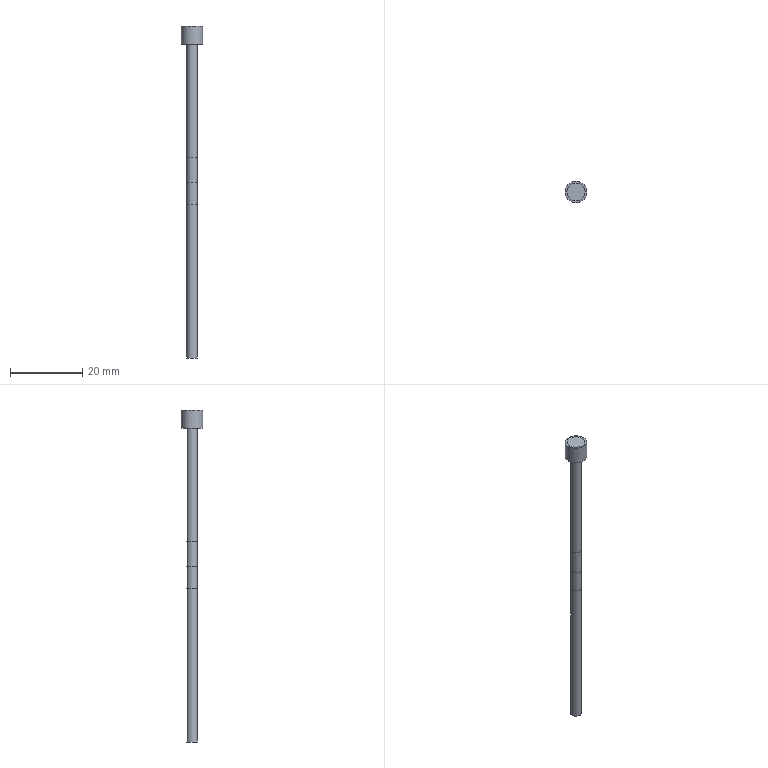Part | NX | features BREP 3 | 3 solids | 17 faces | box 6 x 6 x 92.2 mm | volume 1282 mm3 | plane 9 | cylinder 7 | torus 1 | commonest cylinder face diameters 3 x3 2 x1 2.1 x1 5 x1 6 x1
STEP:
#1=CARTESIAN_POINT('',(-1.5,0.,15.4));
#2=VERTEX_POINT('',#1);
#3=CARTESIAN_POINT('',(0.,0.,15.4));
#4=DIRECTION('',(0.,0.,-1.));
#5=DIRECTION('',(-1.,0.,0.));
#6=AXIS2_PLACEMENT_3D('',#3,#4,#5);
#7=CIRCLE('',#6,1.5);
#8=EDGE_CURVE('',#2,#2,#7,.T.);
#9=ORIENTED_EDGE('',*,*,#8,.T.);
#10=EDGE_LOOP('',(#9));
#11=FACE_BOUND('',#10,.T.);
#12=CARTESIAN_POINT('',(-1.5,0.,-40.2));
#13=VERTEX_POINT('',#12);
#14=CARTESIAN_POINT('',(0.,0.,-40.2));
#15=DIRECTION('',(0.,0.,-1.));
#16=DIRECTION('',(-1.,0.,0.));
#17=AXIS2_PLACEMENT_3D('',#14,#15,#16);
#18=CIRCLE('',#17,1.5);
#19=EDGE_CURVE('',#13,#13,#18,.T.);
#20=ORIENTED_EDGE('',*,*,#19,.F.);
#21=EDGE_LOOP('',(#20));
#22=FACE_BOUND('',#21,.T.);
#23=CARTESIAN_POINT('',(0.,0.,15.4));
#24=DIRECTION('',(0.,0.,-1.));
#25=DIRECTION('',(1.,0.,0.));
#26=AXIS2_PLACEMENT_3D('',#23,#24,#25);
#27=CYLINDRICAL_SURFACE('',#26,1.5);
#28=ADVANCED_FACE('',(#11,#22),#27,.T.);
#29=ORIENTED_EDGE('',*,*,#8,.F.);
#30=EDGE_LOOP('',(#29));
#31=FACE_BOUND('',#30,.T.);
#32=CARTESIAN_POINT('',(0.,0.,15.4));
#33=DIRECTION('',(0.,0.,-1.));
#34=DIRECTION('',(1.,0.,0.));
#35=AXIS2_PLACEMENT_3D('',#32,#33,#34);
#36=PLANE('',#35);
#37=ADVANCED_FACE('',(#31),#36,.F.);
#38=ORIENTED_EDGE('',*,*,#19,.T.);
#39=EDGE_LOOP('',(#38));
#40=FACE_BOUND('',#39,.T.);
#41=CARTESIAN_POINT('',(0.,0.,-40.2));
#42=DIRECTION('',(0.,0.,-1.));
#43=DIRECTION('',(1.,0.,0.));
#44=AXIS2_PLACEMENT_3D('',#41,#42,#43);
#45=PLANE('',#44);
#46=ADVANCED_FACE('',(#40),#45,.T.);
#47=CLOSED_SHELL('',(#28,#37,#46));
#48=MANIFOLD_SOLID_BREP('',#47);
#49=CARTESIAN_POINT('',(2.5,0.,47.));
#50=VERTEX_POINT('',#49);
#51=CARTESIAN_POINT('',(0.,0.,47.));
#52=DIRECTION('',(0.,0.,-1.));
#53=DIRECTION('',(1.,0.,0.));
#54=AXIS2_PLACEMENT_3D('',#51,#52,#53);
#55=CIRCLE('',#54,2.5);
#56=EDGE_CURVE('',#50,#50,#55,.T.);
#57=ORIENTED_EDGE('',*,*,#56,.F.);
#58=EDGE_LOOP('',(#57));
#59=FACE_BOUND('',#58,.T.);
#60=CARTESIAN_POINT('',(2.5,0.,52.));
#61=VERTEX_POINT('',#60);
#62=CARTESIAN_POINT('',(0.,0.,52.));
#63=DIRECTION('',(0.,0.,-1.));
#64=DIRECTION('',(1.,0.,0.));
#65=AXIS2_PLACEMENT_3D('',#62,#63,#64);
#66=CIRCLE('',#65,2.5);
#67=EDGE_CURVE('',#61,#61,#66,.T.);
#68=ORIENTED_EDGE('',*,*,#67,.T.);
#69=EDGE_LOOP('',(#68));
#70=FACE_BOUND('',#69,.T.);
#71=CARTESIAN_POINT('',(0.,0.,47.));
#72=DIRECTION('',(0.,0.,1.));
#73=DIRECTION('',(-1.,0.,0.));
#74=AXIS2_PLACEMENT_3D('',#71,#72,#73);
#75=CYLINDRICAL_SURFACE('',#74,2.5);
#76=ADVANCED_FACE('',(#59,#70),#75,.T.);
#77=CARTESIAN_POINT('',(-1.5,0.,47.));
#78=VERTEX_POINT('',#77);
#79=CARTESIAN_POINT('',(0.,0.,47.));
#80=DIRECTION('',(0.,0.,-1.));
#81=DIRECTION('',(-1.,0.,0.));
#82=AXIS2_PLACEMENT_3D('',#79,#80,#81);
#83=CIRCLE('',#82,1.5);
#84=EDGE_CURVE('',#78,#78,#83,.T.);
#85=ORIENTED_EDGE('',*,*,#84,.F.);
#86=EDGE_LOOP('',(#85));
#87=FACE_BOUND('',#86,.T.);
#88=ORIENTED_EDGE('',*,*,#56,.T.);
#89=EDGE_LOOP('',(#88));
#90=FACE_BOUND('',#89,.T.);
#91=CARTESIAN_POINT('',(0.,0.,47.));
#92=DIRECTION('',(0.,0.,-1.));
#93=DIRECTION('',(1.,0.,0.));
#94=AXIS2_PLACEMENT_3D('',#91,#92,#93);
#95=PLANE('',#94);
#96=ADVANCED_FACE('',(#87,#90),#95,.T.);
#97=ORIENTED_EDGE('',*,*,#67,.F.);
#98=EDGE_LOOP('',(#97));
#99=FACE_BOUND('',#98,.T.);
#100=CARTESIAN_POINT('',(0.,0.,52.));
#101=DIRECTION('',(0.,0.,-1.));
#102=DIRECTION('',(1.,0.,0.));
#103=AXIS2_PLACEMENT_3D('',#100,#101,#102);
#104=PLANE('',#103);
#105=ADVANCED_FACE('',(#99),#104,.F.);
#106=ORIENTED_EDGE('',*,*,#84,.T.);
#107=EDGE_LOOP('',(#106));
#108=FACE_BOUND('',#107,.T.);
#109=CARTESIAN_POINT('',(-1.5,0.,8.522));
#110=VERTEX_POINT('',#109);
#111=CARTESIAN_POINT('',(0.,0.,8.522));
#112=DIRECTION('',(0.,0.,-1.));
#113=DIRECTION('',(-1.,0.,0.));
#114=AXIS2_PLACEMENT_3D('',#111,#112,#113);
#115=CIRCLE('',#114,1.5);
#116=EDGE_CURVE('',#110,#110,#115,.T.);
#117=ORIENTED_EDGE('',*,*,#116,.F.);
#118=EDGE_LOOP('',(#117));
#119=FACE_BOUND('',#118,.T.);
#120=CARTESIAN_POINT('',(0.,0.,47.));
#121=DIRECTION('',(0.,0.,-1.));
#122=DIRECTION('',(1.,0.,0.));
#123=AXIS2_PLACEMENT_3D('',#120,#121,#122);
#124=CYLINDRICAL_SURFACE('',#123,1.5);
#125=ADVANCED_FACE('',(#108,#119),#124,.T.);
#126=ORIENTED_EDGE('',*,*,#116,.T.);
#127=EDGE_LOOP('',(#126));
#128=FACE_BOUND('',#127,.T.);
#129=CARTESIAN_POINT('',(-1.,0.,5.4));
#130=VERTEX_POINT('',#129);
#131=CARTESIAN_POINT('',(0.,0.,5.4));
#132=DIRECTION('',(0.,0.,-1.));
#133=DIRECTION('',(-1.,0.,0.));
#134=AXIS2_PLACEMENT_3D('',#131,#132,#133);
#135=CIRCLE('',#134,1.);
#136=EDGE_CURVE('',#130,#130,#135,.T.);
#137=ORIENTED_EDGE('',*,*,#136,.F.);
#138=EDGE_LOOP('',(#137));
#139=FACE_BOUND('',#138,.T.);
#140=CARTESIAN_POINT('',(0.,0.,5.4));
#141=DIRECTION('',(0.,0.,-1.));
#142=DIRECTION('',(1.,0.,0.));
#143=AXIS2_PLACEMENT_3D('',#140,#141,#142);
#144=TOROIDAL_SURFACE('',#143,11.,10.);
#145=ADVANCED_FACE('',(#128,#139),#144,.F.);
#146=ORIENTED_EDGE('',*,*,#136,.T.);
#147=EDGE_LOOP('',(#146));
#148=FACE_BOUND('',#147,.T.);
#149=CARTESIAN_POINT('',(1.,0.,-3.6));
#150=VERTEX_POINT('',#149);
#151=CARTESIAN_POINT('',(0.,0.,-3.6));
#152=DIRECTION('',(0.,0.,1.));
#153=DIRECTION('',(1.,0.,0.));
#154=AXIS2_PLACEMENT_3D('',#151,#152,#153);
#155=CIRCLE('',#154,1.);
#156=EDGE_CURVE('',#150,#150,#155,.T.);
#157=ORIENTED_EDGE('',*,*,#156,.T.);
#158=EDGE_LOOP('',(#157));
#159=FACE_BOUND('',#158,.T.);
#160=CARTESIAN_POINT('',(0.,0.,0.));
#161=DIRECTION('',(0.,0.,1.));
#162=DIRECTION('',(-1.,0.,0.));
#163=AXIS2_PLACEMENT_3D('',#160,#161,#162);
#164=CYLINDRICAL_SURFACE('',#163,1.);
#165=ADVANCED_FACE('',(#148,#159),#164,.T.);
#166=ORIENTED_EDGE('',*,*,#156,.F.);
#167=EDGE_LOOP('',(#166));
#168=FACE_BOUND('',#167,.T.);
#169=CARTESIAN_POINT('',(5.458,-13.172,-3.6));
#170=DIRECTION('',(0.,0.,1.));
#171=DIRECTION('',(-1.,0.,0.));
#172=AXIS2_PLACEMENT_3D('',#169,#170,#171);
#173=PLANE('',#172);
#174=ADVANCED_FACE('',(#168),#173,.F.);
#175=CLOSED_SHELL('',(#76,#96,#105,#125,#145,#165,#174));
#176=MANIFOLD_SOLID_BREP('',#175);
#177=CARTESIAN_POINT('',(3.,0.,47.));
#178=VERTEX_POINT('',#177);
#179=CARTESIAN_POINT('',(0.,0.,47.));
#180=DIRECTION('',(0.,0.,-1.));
#181=DIRECTION('',(1.,0.,0.));
#182=AXIS2_PLACEMENT_3D('',#179,#180,#181);
#183=CIRCLE('',#182,3.);
#184=EDGE_CURVE('',#178,#178,#183,.T.);
#185=ORIENTED_EDGE('',*,*,#184,.F.);
#186=EDGE_LOOP('',(#185));
#187=FACE_BOUND('',#186,.T.);
#188=CARTESIAN_POINT('',(3.,0.,52.));
#189=VERTEX_POINT('',#188);
#190=CARTESIAN_POINT('',(0.,0.,52.));
#191=DIRECTION('',(0.,0.,-1.));
#192=DIRECTION('',(1.,0.,0.));
#193=AXIS2_PLACEMENT_3D('',#190,#191,#192);
#194=CIRCLE('',#193,3.);
#195=EDGE_CURVE('',#189,#189,#194,.T.);
#196=ORIENTED_EDGE('',*,*,#195,.T.);
#197=EDGE_LOOP('',(#196));
#198=FACE_BOUND('',#197,.T.);
#199=CARTESIAN_POINT('',(0.,0.,47.));
#200=DIRECTION('',(0.,0.,1.));
#201=DIRECTION('',(-1.,0.,0.));
#202=AXIS2_PLACEMENT_3D('',#199,#200,#201);
#203=CYLINDRICAL_SURFACE('',#202,3.);
#204=ADVANCED_FACE('',(#187,#198),#203,.T.);
#205=CARTESIAN_POINT('',(-1.5,0.,47.));
#206=VERTEX_POINT('',#205);
#207=CARTESIAN_POINT('',(0.,0.,47.));
#208=DIRECTION('',(0.,0.,-1.));
#209=DIRECTION('',(-1.,0.,0.));
#210=AXIS2_PLACEMENT_3D('',#207,#208,#209);
#211=CIRCLE('',#210,1.5);
#212=EDGE_CURVE('',#206,#206,#211,.T.);
#213=ORIENTED_EDGE('',*,*,#212,.F.);
#214=EDGE_LOOP('',(#213));
#215=FACE_BOUND('',#214,.T.);
#216=ORIENTED_EDGE('',*,*,#184,.T.);
#217=EDGE_LOOP('',(#216));
#218=FACE_BOUND('',#217,.T.);
#219=CARTESIAN_POINT('',(0.,0.,47.));
#220=DIRECTION('',(0.,0.,-1.));
#221=DIRECTION('',(1.,0.,0.));
#222=AXIS2_PLACEMENT_3D('',#219,#220,#221);
#223=PLANE('',#222);
#224=ADVANCED_FACE('',(#215,#218),#223,.T.);
#225=ORIENTED_EDGE('',*,*,#195,.F.);
#226=EDGE_LOOP('',(#225));
#227=FACE_BOUND('',#226,.T.);
#228=CARTESIAN_POINT('',(0.,0.,52.));
#229=DIRECTION('',(0.,0.,-1.));
#230=DIRECTION('',(1.,0.,0.));
#231=AXIS2_PLACEMENT_3D('',#228,#229,#230);
#232=PLANE('',#231);
#233=ADVANCED_FACE('',(#227),#232,.F.);
#234=CARTESIAN_POINT('',(1.05,0.,2.4));
#235=VERTEX_POINT('',#234);
#236=CARTESIAN_POINT('',(0.,0.,2.4));
#237=DIRECTION('',(0.,0.,1.));
#238=DIRECTION('',(1.,0.,0.));
#239=AXIS2_PLACEMENT_3D('',#236,#237,#238);
#240=CIRCLE('',#239,1.05);
#241=EDGE_CURVE('',#235,#235,#240,.T.);
#242=ORIENTED_EDGE('',*,*,#241,.T.);
#243=EDGE_LOOP('',(#242));
#244=FACE_BOUND('',#243,.T.);
#245=CARTESIAN_POINT('',(-1.5,0.,2.4));
#246=VERTEX_POINT('',#245);
#247=CARTESIAN_POINT('',(0.,0.,2.4));
#248=DIRECTION('',(0.,0.,-1.));
#249=DIRECTION('',(-1.,0.,0.));
#250=AXIS2_PLACEMENT_3D('',#247,#248,#249);
#251=CIRCLE('',#250,1.5);
#252=EDGE_CURVE('',#246,#246,#251,.T.);
#253=ORIENTED_EDGE('',*,*,#252,.T.);
#254=EDGE_LOOP('',(#253));
#255=FACE_BOUND('',#254,.T.);
#256=CARTESIAN_POINT('',(0.,0.,2.4));
#257=DIRECTION('',(0.,0.,-1.));
#258=DIRECTION('',(1.,0.,0.));
#259=AXIS2_PLACEMENT_3D('',#256,#257,#258);
#260=PLANE('',#259);
#261=ADVANCED_FACE('',(#244,#255),#260,.T.);
#262=ORIENTED_EDGE('',*,*,#252,.F.);
#263=EDGE_LOOP('',(#262));
#264=FACE_BOUND('',#263,.T.);
#265=ORIENTED_EDGE('',*,*,#212,.T.);
#266=EDGE_LOOP('',(#265));
#267=FACE_BOUND('',#266,.T.);
#268=CARTESIAN_POINT('',(0.,0.,47.));
#269=DIRECTION('',(0.,0.,-1.));
#270=DIRECTION('',(1.,0.,0.));
#271=AXIS2_PLACEMENT_3D('',#268,#269,#270);
#272=CYLINDRICAL_SURFACE('',#271,1.5);
#273=ADVANCED_FACE('',(#264,#267),#272,.T.);
#274=CARTESIAN_POINT('',(1.05,0.,-3.6));
#275=VERTEX_POINT('',#274);
#276=CARTESIAN_POINT('',(0.,0.,-3.6));
#277=DIRECTION('',(0.,0.,1.));
#278=DIRECTION('',(1.,0.,0.));
#279=AXIS2_PLACEMENT_3D('',#276,#277,#278);
#280=CIRCLE('',#279,1.05);
#281=EDGE_CURVE('',#275,#275,#280,.T.);
#282=ORIENTED_EDGE('',*,*,#281,.T.);
#283=EDGE_LOOP('',(#282));
#284=FACE_BOUND('',#283,.T.);
#285=ORIENTED_EDGE('',*,*,#241,.F.);
#286=EDGE_LOOP('',(#285));
#287=FACE_BOUND('',#286,.T.);
#288=CARTESIAN_POINT('',(0.,0.,0.));
#289=DIRECTION('',(0.,0.,1.));
#290=DIRECTION('',(-1.,0.,0.));
#291=AXIS2_PLACEMENT_3D('',#288,#289,#290);
#292=CYLINDRICAL_SURFACE('',#291,1.05);
#293=ADVANCED_FACE('',(#284,#287),#292,.T.);
#294=ORIENTED_EDGE('',*,*,#281,.F.);
#295=EDGE_LOOP('',(#294));
#296=FACE_BOUND('',#295,.T.);
#297=CARTESIAN_POINT('',(5.458,-13.172,-3.6));
#298=DIRECTION('',(0.,0.,1.));
#299=DIRECTION('',(-1.,0.,0.));
#300=AXIS2_PLACEMENT_3D('',#297,#298,#299);
#301=PLANE('',#300);
#302=ADVANCED_FACE('',(#296),#301,.F.);
#303=CLOSED_SHELL('',(#204,#224,#233,#261,#273,#293,#302));
#304=MANIFOLD_SOLID_BREP('',#303);
#305=(LENGTH_UNIT()NAMED_UNIT(*)SI_UNIT(.MILLI.,.METRE.));
#306=UNCERTAINTY_MEASURE_WITH_UNIT(LENGTH_MEASURE(0.00001),#305,'','');
#307=(NAMED_UNIT(*)PLANE_ANGLE_UNIT()SI_UNIT($,.RADIAN.));
#308=(NAMED_UNIT(*)SI_UNIT($,.STERADIAN.)SOLID_ANGLE_UNIT());
#309=(GEOMETRIC_REPRESENTATION_CONTEXT(3)GLOBAL_UNCERTAINTY_ASSIGNED_CONTEXT((#306))GLOBAL_UNIT_ASSIGNED_CONTEXT((#305,#307,#308))REPRESENTATION_CONTEXT('',''));
#310=ADVANCED_BREP_SHAPE_REPRESENTATION('',(#48,#176,#304),#309);